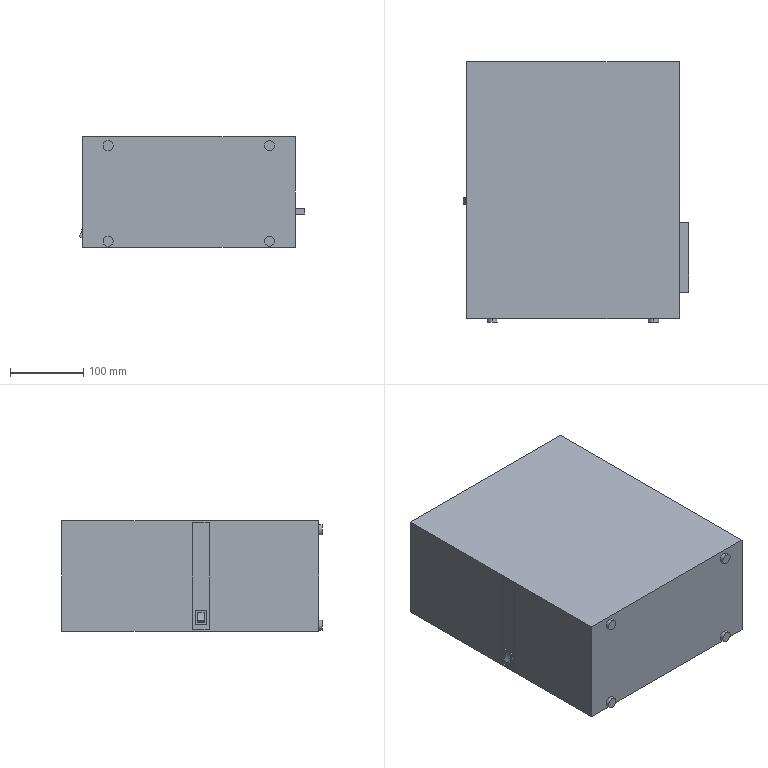Part | SolidWorks | features ICE 5, Extrusion 1 | 1 solid | 37 faces | box 307.5 x 355 x 150 mm | volume 15234035 mm3 | plane 28 | cylinder 9 | commonest cylinder face diameters 14 x8 44 x1
STEP:
#1=CARTESIAN_POINT('',(-110.,-5.,-74.));
#2=VERTEX_POINT('',#1);
#3=CARTESIAN_POINT('',(-110.,-5.,-60.));
#4=VERTEX_POINT('',#3);
#5=CARTESIAN_POINT('',(-110.,-5.,-67.));
#6=DIRECTION('',(0.,-1.,0.));
#7=DIRECTION('',(0.,0.,1.));
#8=AXIS2_PLACEMENT_3D('',#5,#6,#7);
#9=CIRCLE('',#8,7.);
#10=EDGE_CURVE('',#2,#4,#9,.T.);
#11=ORIENTED_EDGE('',*,*,#10,.F.);
#12=CARTESIAN_POINT('',(-110.,0.,-74.));
#13=VERTEX_POINT('',#12);
#14=CARTESIAN_POINT('',(-110.,-5.,-74.));
#15=DIRECTION('',(0.,1.,0.));
#16=VECTOR('',#15,1000.);
#17=LINE('',#14,#16);
#18=EDGE_CURVE('',#2,#13,#17,.T.);
#19=ORIENTED_EDGE('',*,*,#18,.T.);
#20=CARTESIAN_POINT('',(-110.,0.,-60.));
#21=VERTEX_POINT('',#20);
#22=CARTESIAN_POINT('',(-110.,0.,-67.));
#23=DIRECTION('',(0.,-1.,0.));
#24=DIRECTION('',(0.,0.,1.));
#25=AXIS2_PLACEMENT_3D('',#22,#23,#24);
#26=CIRCLE('',#25,7.);
#27=EDGE_CURVE('',#13,#21,#26,.T.);
#28=ORIENTED_EDGE('',*,*,#27,.T.);
#29=CARTESIAN_POINT('',(-110.,-5.,-60.));
#30=DIRECTION('',(0.,1.,0.));
#31=VECTOR('',#30,1000.);
#32=LINE('',#29,#31);
#33=EDGE_CURVE('',#4,#21,#32,.T.);
#34=ORIENTED_EDGE('',*,*,#33,.F.);
#35=EDGE_LOOP('',(#11,#19,#28,#34));
#36=FACE_OUTER_BOUND('',#35,.T.);
#37=CARTESIAN_POINT('',(-110.,-5.,-67.));
#38=DIRECTION('',(0.,1.,0.));
#39=DIRECTION('',(0.,0.,1.));
#40=AXIS2_PLACEMENT_3D('',#37,#38,#39);
#41=CYLINDRICAL_SURFACE('',#40,7.);
#42=ADVANCED_FACE('',(#36),#41,.T.);
#43=CARTESIAN_POINT('',(110.,-5.,-74.));
#44=VERTEX_POINT('',#43);
#45=CARTESIAN_POINT('',(110.,-5.,-60.));
#46=VERTEX_POINT('',#45);
#47=CARTESIAN_POINT('',(110.,-5.,-67.));
#48=DIRECTION('',(0.,-1.,0.));
#49=DIRECTION('',(0.,0.,-1.));
#50=AXIS2_PLACEMENT_3D('',#47,#48,#49);
#51=CIRCLE('',#50,7.);
#52=EDGE_CURVE('',#44,#46,#51,.T.);
#53=ORIENTED_EDGE('',*,*,#52,.F.);
#54=CARTESIAN_POINT('',(110.,0.,-74.));
#55=VERTEX_POINT('',#54);
#56=CARTESIAN_POINT('',(110.,-5.,-74.));
#57=DIRECTION('',(0.,1.,0.));
#58=VECTOR('',#57,1000.);
#59=LINE('',#56,#58);
#60=EDGE_CURVE('',#44,#55,#59,.T.);
#61=ORIENTED_EDGE('',*,*,#60,.T.);
#62=CARTESIAN_POINT('',(110.,0.,-60.));
#63=VERTEX_POINT('',#62);
#64=CARTESIAN_POINT('',(110.,0.,-67.));
#65=DIRECTION('',(0.,-1.,0.));
#66=DIRECTION('',(0.,0.,1.));
#67=AXIS2_PLACEMENT_3D('',#64,#65,#66);
#68=CIRCLE('',#67,7.);
#69=EDGE_CURVE('',#55,#63,#68,.T.);
#70=ORIENTED_EDGE('',*,*,#69,.T.);
#71=CARTESIAN_POINT('',(110.,-5.,-60.));
#72=DIRECTION('',(0.,1.,0.));
#73=VECTOR('',#72,1000.);
#74=LINE('',#71,#73);
#75=EDGE_CURVE('',#46,#63,#74,.T.);
#76=ORIENTED_EDGE('',*,*,#75,.F.);
#77=EDGE_LOOP('',(#53,#61,#70,#76));
#78=FACE_OUTER_BOUND('',#77,.T.);
#79=CARTESIAN_POINT('',(110.,-5.,-67.));
#80=DIRECTION('',(0.,1.,0.));
#81=DIRECTION('',(0.,0.,1.));
#82=AXIS2_PLACEMENT_3D('',#79,#80,#81);
#83=CYLINDRICAL_SURFACE('',#82,7.);
#84=ADVANCED_FACE('',(#78),#83,.T.);
#85=CARTESIAN_POINT('',(110.,-5.,56.));
#86=VERTEX_POINT('',#85);
#87=CARTESIAN_POINT('',(110.,-5.,70.));
#88=VERTEX_POINT('',#87);
#89=CARTESIAN_POINT('',(110.,-5.,63.));
#90=DIRECTION('',(0.,-1.,0.));
#91=DIRECTION('',(0.,0.,1.));
#92=AXIS2_PLACEMENT_3D('',#89,#90,#91);
#93=CIRCLE('',#92,7.);
#94=EDGE_CURVE('',#86,#88,#93,.T.);
#95=ORIENTED_EDGE('',*,*,#94,.F.);
#96=CARTESIAN_POINT('',(110.,0.,56.));
#97=VERTEX_POINT('',#96);
#98=CARTESIAN_POINT('',(110.,-5.,56.));
#99=DIRECTION('',(0.,1.,0.));
#100=VECTOR('',#99,1000.);
#101=LINE('',#98,#100);
#102=EDGE_CURVE('',#86,#97,#101,.T.);
#103=ORIENTED_EDGE('',*,*,#102,.T.);
#104=CARTESIAN_POINT('',(110.,0.,70.));
#105=VERTEX_POINT('',#104);
#106=CARTESIAN_POINT('',(110.,0.,63.));
#107=DIRECTION('',(0.,-1.,0.));
#108=DIRECTION('',(0.,0.,1.));
#109=AXIS2_PLACEMENT_3D('',#106,#107,#108);
#110=CIRCLE('',#109,7.);
#111=EDGE_CURVE('',#97,#105,#110,.T.);
#112=ORIENTED_EDGE('',*,*,#111,.T.);
#113=CARTESIAN_POINT('',(110.,-5.,70.));
#114=DIRECTION('',(0.,1.,0.));
#115=VECTOR('',#114,1000.);
#116=LINE('',#113,#115);
#117=EDGE_CURVE('',#88,#105,#116,.T.);
#118=ORIENTED_EDGE('',*,*,#117,.F.);
#119=EDGE_LOOP('',(#95,#103,#112,#118));
#120=FACE_OUTER_BOUND('',#119,.T.);
#121=CARTESIAN_POINT('',(110.,-5.,63.));
#122=DIRECTION('',(0.,1.,0.));
#123=DIRECTION('',(0.,0.,1.));
#124=AXIS2_PLACEMENT_3D('',#121,#122,#123);
#125=CYLINDRICAL_SURFACE('',#124,7.);
#126=ADVANCED_FACE('',(#120),#125,.T.);
#127=CARTESIAN_POINT('',(-110.,-5.,56.));
#128=VERTEX_POINT('',#127);
#129=CARTESIAN_POINT('',(-110.,-5.,70.));
#130=VERTEX_POINT('',#129);
#131=CARTESIAN_POINT('',(-110.,-5.,63.));
#132=DIRECTION('',(0.,-1.,0.));
#133=DIRECTION('',(0.,0.,-1.));
#134=AXIS2_PLACEMENT_3D('',#131,#132,#133);
#135=CIRCLE('',#134,7.);
#136=EDGE_CURVE('',#128,#130,#135,.T.);
#137=ORIENTED_EDGE('',*,*,#136,.F.);
#138=CARTESIAN_POINT('',(-110.,0.,56.));
#139=VERTEX_POINT('',#138);
#140=CARTESIAN_POINT('',(-110.,-5.,56.));
#141=DIRECTION('',(0.,1.,0.));
#142=VECTOR('',#141,1000.);
#143=LINE('',#140,#142);
#144=EDGE_CURVE('',#128,#139,#143,.T.);
#145=ORIENTED_EDGE('',*,*,#144,.T.);
#146=CARTESIAN_POINT('',(-110.,0.,70.));
#147=VERTEX_POINT('',#146);
#148=CARTESIAN_POINT('',(-110.,0.,63.));
#149=DIRECTION('',(0.,-1.,0.));
#150=DIRECTION('',(0.,0.,1.));
#151=AXIS2_PLACEMENT_3D('',#148,#149,#150);
#152=CIRCLE('',#151,7.);
#153=EDGE_CURVE('',#139,#147,#152,.T.);
#154=ORIENTED_EDGE('',*,*,#153,.T.);
#155=CARTESIAN_POINT('',(-110.,-5.,70.));
#156=DIRECTION('',(0.,1.,0.));
#157=VECTOR('',#156,1000.);
#158=LINE('',#155,#157);
#159=EDGE_CURVE('',#130,#147,#158,.T.);
#160=ORIENTED_EDGE('',*,*,#159,.F.);
#161=EDGE_LOOP('',(#137,#145,#154,#160));
#162=FACE_OUTER_BOUND('',#161,.T.);
#163=CARTESIAN_POINT('',(-110.,-5.,63.));
#164=DIRECTION('',(0.,1.,0.));
#165=DIRECTION('',(0.,0.,1.));
#166=AXIS2_PLACEMENT_3D('',#163,#164,#165);
#167=CYLINDRICAL_SURFACE('',#166,7.);
#168=ADVANCED_FACE('',(#162),#167,.T.);
#169=CARTESIAN_POINT('',(145.,0.,75.));
#170=VERTEX_POINT('',#169);
#171=CARTESIAN_POINT('',(145.,0.,-75.));
#172=VERTEX_POINT('',#171);
#173=CARTESIAN_POINT('',(145.,0.,75.));
#174=DIRECTION('',(0.,0.,-1.));
#175=VECTOR('',#174,1000.);
#176=LINE('',#173,#175);
#177=EDGE_CURVE('',#170,#172,#176,.T.);
#178=ORIENTED_EDGE('',*,*,#177,.T.);
#179=CARTESIAN_POINT('',(145.,350.,-75.));
#180=VERTEX_POINT('',#179);
#181=CARTESIAN_POINT('',(145.,350.,-75.));
#182=DIRECTION('',(0.,-1.,0.));
#183=VECTOR('',#182,1000.);
#184=LINE('',#181,#183);
#185=EDGE_CURVE('',#180,#172,#184,.T.);
#186=ORIENTED_EDGE('',*,*,#185,.F.);
#187=CARTESIAN_POINT('',(145.,350.,75.));
#188=VERTEX_POINT('',#187);
#189=CARTESIAN_POINT('',(145.,350.,75.));
#190=DIRECTION('',(0.,0.,-1.));
#191=VECTOR('',#190,1000.);
#192=LINE('',#189,#191);
#193=EDGE_CURVE('',#188,#180,#192,.T.);
#194=ORIENTED_EDGE('',*,*,#193,.F.);
#195=CARTESIAN_POINT('',(145.,350.,75.));
#196=DIRECTION('',(0.,-1.,0.));
#197=VECTOR('',#196,1000.);
#198=LINE('',#195,#197);
#199=EDGE_CURVE('',#188,#170,#198,.T.);
#200=ORIENTED_EDGE('',*,*,#199,.T.);
#201=EDGE_LOOP('',(#178,#186,#194,#200));
#202=FACE_OUTER_BOUND('',#201,.T.);
#203=CARTESIAN_POINT('',(145.,131.,-23.));
#204=VERTEX_POINT('',#203);
#205=CARTESIAN_POINT('',(145.,36.,-23.));
#206=VERTEX_POINT('',#205);
#207=CARTESIAN_POINT('',(145.,36.,-23.));
#208=DIRECTION('',(0.,-1.,0.));
#209=VECTOR('',#208,1000.);
#210=LINE('',#207,#209);
#211=EDGE_CURVE('',#204,#206,#210,.T.);
#212=ORIENTED_EDGE('',*,*,#211,.F.);
#213=CARTESIAN_POINT('',(145.,131.,-30.));
#214=VERTEX_POINT('',#213);
#215=CARTESIAN_POINT('',(145.,131.,-30.));
#216=DIRECTION('',(0.,0.,1.));
#217=VECTOR('',#216,1000.);
#218=LINE('',#215,#217);
#219=EDGE_CURVE('',#214,#204,#218,.T.);
#220=ORIENTED_EDGE('',*,*,#219,.F.);
#221=CARTESIAN_POINT('',(145.,36.,-30.));
#222=VERTEX_POINT('',#221);
#223=CARTESIAN_POINT('',(145.,36.,-30.));
#224=DIRECTION('',(0.,1.,0.));
#225=VECTOR('',#224,1000.);
#226=LINE('',#223,#225);
#227=EDGE_CURVE('',#222,#214,#226,.T.);
#228=ORIENTED_EDGE('',*,*,#227,.F.);
#229=CARTESIAN_POINT('',(145.,36.,-30.));
#230=DIRECTION('',(0.,0.,-1.));
#231=VECTOR('',#230,1000.);
#232=LINE('',#229,#231);
#233=EDGE_CURVE('',#206,#222,#232,.T.);
#234=ORIENTED_EDGE('',*,*,#233,.F.);
#235=EDGE_LOOP('',(#212,#220,#228,#234));
#236=FACE_BOUND('',#235,.T.);
#237=CARTESIAN_POINT('',(145.,350.,75.));
#238=DIRECTION('',(-1.,0.,0.));
#239=DIRECTION('',(0.,0.,1.));
#240=AXIS2_PLACEMENT_3D('',#237,#238,#239);
#241=PLANE('',#240);
#242=ADVANCED_FACE('',(#202,#236),#241,.F.);
#243=CARTESIAN_POINT('',(-145.5,168.,-66.5));
#244=VERTEX_POINT('',#243);
#245=CARTESIAN_POINT('',(-145.5,153.,-66.5));
#246=VERTEX_POINT('',#245);
#247=CARTESIAN_POINT('',(-145.5,153.,-66.5));
#248=DIRECTION('',(0.,-1.,0.));
#249=VECTOR('',#248,1000.);
#250=LINE('',#247,#249);
#251=EDGE_CURVE('',#244,#246,#250,.T.);
#252=ORIENTED_EDGE('',*,*,#251,.T.);
#253=CARTESIAN_POINT('',(-145.5,153.,-46.5));
#254=VERTEX_POINT('',#253);
#255=CARTESIAN_POINT('',(-145.5,153.,-46.5));
#256=DIRECTION('',(0.,0.,1.));
#257=VECTOR('',#256,1000.);
#258=LINE('',#255,#257);
#259=EDGE_CURVE('',#246,#254,#258,.T.);
#260=ORIENTED_EDGE('',*,*,#259,.T.);
#261=CARTESIAN_POINT('',(-145.5,168.,-46.5));
#262=VERTEX_POINT('',#261);
#263=CARTESIAN_POINT('',(-145.5,153.,-46.5));
#264=DIRECTION('',(0.,1.,0.));
#265=VECTOR('',#264,1000.);
#266=LINE('',#263,#265);
#267=EDGE_CURVE('',#254,#262,#266,.T.);
#268=ORIENTED_EDGE('',*,*,#267,.T.);
#269=CARTESIAN_POINT('',(-145.5,168.,-46.5));
#270=DIRECTION('',(0.,0.,-1.));
#271=VECTOR('',#270,1000.);
#272=LINE('',#269,#271);
#273=EDGE_CURVE('',#262,#244,#272,.T.);
#274=ORIENTED_EDGE('',*,*,#273,.T.);
#275=EDGE_LOOP('',(#252,#260,#268,#274));
#276=FACE_OUTER_BOUND('',#275,.T.);
#277=CARTESIAN_POINT('',(-145.5,156.,-49.5));
#278=VERTEX_POINT('',#277);
#279=CARTESIAN_POINT('',(-145.5,165.,-49.5));
#280=VERTEX_POINT('',#279);
#281=CARTESIAN_POINT('',(-145.5,156.,-49.5));
#282=DIRECTION('',(0.,1.,0.));
#283=VECTOR('',#282,1000.);
#284=LINE('',#281,#283);
#285=EDGE_CURVE('',#278,#280,#284,.T.);
#286=ORIENTED_EDGE('',*,*,#285,.F.);
#287=CARTESIAN_POINT('',(-145.5,156.,-63.5));
#288=VERTEX_POINT('',#287);
#289=CARTESIAN_POINT('',(-145.5,156.,-63.5));
#290=DIRECTION('',(0.,0.,1.));
#291=VECTOR('',#290,1000.);
#292=LINE('',#289,#291);
#293=EDGE_CURVE('',#288,#278,#292,.T.);
#294=ORIENTED_EDGE('',*,*,#293,.F.);
#295=CARTESIAN_POINT('',(-145.5,165.,-63.5));
#296=VERTEX_POINT('',#295);
#297=CARTESIAN_POINT('',(-145.5,156.,-63.5));
#298=DIRECTION('',(0.,1.,0.));
#299=VECTOR('',#298,1000.);
#300=LINE('',#297,#299);
#301=EDGE_CURVE('',#288,#296,#300,.T.);
#302=ORIENTED_EDGE('',*,*,#301,.T.);
#303=CARTESIAN_POINT('',(-145.5,165.,-63.5));
#304=DIRECTION('',(0.,0.,1.));
#305=VECTOR('',#304,1000.);
#306=LINE('',#303,#305);
#307=EDGE_CURVE('',#296,#280,#306,.T.);
#308=ORIENTED_EDGE('',*,*,#307,.T.);
#309=EDGE_LOOP('',(#286,#294,#302,#308));
#310=FACE_BOUND('',#309,.T.);
#311=CARTESIAN_POINT('',(-145.5,0.,0.));
#312=DIRECTION('',(-1.,0.,0.));
#313=DIRECTION('',(0.,0.,1.));
#314=AXIS2_PLACEMENT_3D('',#311,#312,#313);
#315=PLANE('',#314);
#316=ADVANCED_FACE('',(#276,#310),#315,.T.);
#317=CARTESIAN_POINT('',(-144.,172.,-72.5));
#318=VERTEX_POINT('',#317);
#319=CARTESIAN_POINT('',(-144.,149.,-72.5));
#320=VERTEX_POINT('',#319);
#321=CARTESIAN_POINT('',(-144.,149.,-72.5));
#322=DIRECTION('',(0.,-1.,0.));
#323=VECTOR('',#322,1000.);
#324=LINE('',#321,#323);
#325=EDGE_CURVE('',#318,#320,#324,.T.);
#326=ORIENTED_EDGE('',*,*,#325,.T.);
#327=CARTESIAN_POINT('',(-144.,149.,72.5));
#328=VERTEX_POINT('',#327);
#329=CARTESIAN_POINT('',(-144.,149.,72.5));
#330=DIRECTION('',(0.,0.,1.));
#331=VECTOR('',#330,1000.);
#332=LINE('',#329,#331);
#333=EDGE_CURVE('',#320,#328,#332,.T.);
#334=ORIENTED_EDGE('',*,*,#333,.T.);
#335=CARTESIAN_POINT('',(-144.,172.,72.5));
#336=VERTEX_POINT('',#335);
#337=CARTESIAN_POINT('',(-144.,149.,72.5));
#338=DIRECTION('',(0.,1.,0.));
#339=VECTOR('',#338,1000.);
#340=LINE('',#337,#339);
#341=EDGE_CURVE('',#328,#336,#340,.T.);
#342=ORIENTED_EDGE('',*,*,#341,.T.);
#343=CARTESIAN_POINT('',(-144.,172.,72.5));
#344=DIRECTION('',(0.,0.,-1.));
#345=VECTOR('',#344,1000.);
#346=LINE('',#343,#345);
#347=EDGE_CURVE('',#336,#318,#346,.T.);
#348=ORIENTED_EDGE('',*,*,#347,.T.);
#349=EDGE_LOOP('',(#326,#334,#342,#348));
#350=FACE_OUTER_BOUND('',#349,.T.);
#351=CARTESIAN_POINT('',(-144.,153.,-66.5));
#352=VERTEX_POINT('',#351);
#353=CARTESIAN_POINT('',(-144.,153.,-46.5));
#354=VERTEX_POINT('',#353);
#355=CARTESIAN_POINT('',(-144.,153.,-46.5));
#356=DIRECTION('',(0.,0.,1.));
#357=VECTOR('',#356,1000.);
#358=LINE('',#355,#357);
#359=EDGE_CURVE('',#352,#354,#358,.T.);
#360=ORIENTED_EDGE('',*,*,#359,.F.);
#361=CARTESIAN_POINT('',(-144.,168.,-66.5));
#362=VERTEX_POINT('',#361);
#363=CARTESIAN_POINT('',(-144.,153.,-66.5));
#364=DIRECTION('',(0.,-1.,0.));
#365=VECTOR('',#364,1000.);
#366=LINE('',#363,#365);
#367=EDGE_CURVE('',#362,#352,#366,.T.);
#368=ORIENTED_EDGE('',*,*,#367,.F.);
#369=CARTESIAN_POINT('',(-144.,168.,-46.5));
#370=VERTEX_POINT('',#369);
#371=CARTESIAN_POINT('',(-144.,168.,-46.5));
#372=DIRECTION('',(0.,0.,-1.));
#373=VECTOR('',#372,1000.);
#374=LINE('',#371,#373);
#375=EDGE_CURVE('',#370,#362,#374,.T.);
#376=ORIENTED_EDGE('',*,*,#375,.F.);
#377=CARTESIAN_POINT('',(-144.,153.,-46.5));
#378=DIRECTION('',(0.,1.,0.));
#379=VECTOR('',#378,1000.);
#380=LINE('',#377,#379);
#381=EDGE_CURVE('',#354,#370,#380,.T.);
#382=ORIENTED_EDGE('',*,*,#381,.F.);
#383=EDGE_LOOP('',(#360,#368,#376,#382));
#384=FACE_BOUND('',#383,.T.);
#385=CARTESIAN_POINT('',(-144.,0.,0.));
#386=DIRECTION('',(-1.,0.,0.));
#387=DIRECTION('',(0.,0.,1.));
#388=AXIS2_PLACEMENT_3D('',#385,#386,#387);
#389=PLANE('',#388);
#390=ADVANCED_FACE('',(#350,#384),#389,.T.);
#391=CARTESIAN_POINT('',(-145.,149.,-72.5));
#392=VERTEX_POINT('',#391);
#393=CARTESIAN_POINT('',(-145.,149.,72.5));
#394=VERTEX_POINT('',#393);
#395=CARTESIAN_POINT('',(-145.,149.,72.5));
#396=DIRECTION('',(0.,0.,1.));
#397=VECTOR('',#396,1000.);
#398=LINE('',#395,#397);
#399=EDGE_CURVE('',#392,#394,#398,.T.);
#400=ORIENTED_EDGE('',*,*,#399,.F.);
#401=CARTESIAN_POINT('',(-145.,172.,-72.5));
#402=VERTEX_POINT('',#401);
#403=CARTESIAN_POINT('',(-145.,149.,-72.5));
#404=DIRECTION('',(0.,-1.,0.));
#405=VECTOR('',#404,1000.);
#406=LINE('',#403,#405);
#407=EDGE_CURVE('',#402,#392,#406,.T.);
#408=ORIENTED_EDGE('',*,*,#407,.F.);
#409=CARTESIAN_POINT('',(-145.,172.,72.5));
#410=VERTEX_POINT('',#409);
#411=CARTESIAN_POINT('',(-145.,172.,72.5));
#412=DIRECTION('',(0.,0.,-1.));
#413=VECTOR('',#412,1000.);
#414=LINE('',#411,#413);
#415=EDGE_CURVE('',#410,#402,#414,.T.);
#416=ORIENTED_EDGE('',*,*,#415,.F.);
#417=CARTESIAN_POINT('',(-145.,149.,72.5));
#418=DIRECTION('',(0.,1.,0.));
#419=VECTOR('',#418,1000.);
#420=LINE('',#417,#419);
#421=EDGE_CURVE('',#394,#410,#420,.T.);
#422=ORIENTED_EDGE('',*,*,#421,.F.);
#423=EDGE_LOOP('',(#400,#408,#416,#422));
#424=FACE_BOUND('',#423,.T.);
#425=CARTESIAN_POINT('',(-145.,0.,-75.));
#426=VERTEX_POINT('',#425);
#427=CARTESIAN_POINT('',(-145.,0.,75.));
#428=VERTEX_POINT('',#427);
#429=CARTESIAN_POINT('',(-145.,0.,75.));
#430=DIRECTION('',(0.,0.,1.));
#431=VECTOR('',#430,1000.);
#432=LINE('',#429,#431);
#433=EDGE_CURVE('',#426,#428,#432,.T.);
#434=ORIENTED_EDGE('',*,*,#433,.T.);
#435=CARTESIAN_POINT('',(-145.,350.,75.));
#436=VERTEX_POINT('',#435);
#437=CARTESIAN_POINT('',(-145.,350.,75.));
#438=DIRECTION('',(0.,-1.,0.));
#439=VECTOR('',#438,1000.);
#440=LINE('',#437,#439);
#441=EDGE_CURVE('',#436,#428,#440,.T.);
#442=ORIENTED_EDGE('',*,*,#441,.F.);
#443=CARTESIAN_POINT('',(-145.,350.,-75.));
#444=VERTEX_POINT('',#443);
#445=CARTESIAN_POINT('',(-145.,350.,75.));
#446=DIRECTION('',(0.,0.,1.));
#447=VECTOR('',#446,1000.);
#448=LINE('',#445,#447);
#449=EDGE_CURVE('',#444,#436,#448,.T.);
#450=ORIENTED_EDGE('',*,*,#449,.F.);
#451=CARTESIAN_POINT('',(-145.,350.,-75.));
#452=DIRECTION('',(0.,-1.,0.));
#453=VECTOR('',#452,1000.);
#454=LINE('',#451,#453);
#455=EDGE_CURVE('',#444,#426,#454,.T.);
#456=ORIENTED_EDGE('',*,*,#455,.T.);
#457=EDGE_LOOP('',(#434,#442,#450,#456));
#458=FACE_OUTER_BOUND('',#457,.T.);
#459=CARTESIAN_POINT('',(-145.,350.,75.));
#460=DIRECTION('',(1.,0.,0.));
#461=DIRECTION('',(0.,0.,-1.));
#462=AXIS2_PLACEMENT_3D('',#459,#460,#461);
#463=PLANE('',#462);
#464=ADVANCED_FACE('',(#424,#458),#463,.F.);
#465=CARTESIAN_POINT('',(145.,0.,75.));
#466=DIRECTION('',(1.,0.,0.));
#467=VECTOR('',#466,1000.);
#468=LINE('',#465,#467);
#469=EDGE_CURVE('',#428,#170,#468,.T.);
#470=ORIENTED_EDGE('',*,*,#469,.T.);
#471=ORIENTED_EDGE('',*,*,#199,.F.);
#472=CARTESIAN_POINT('',(145.,350.,75.));
#473=DIRECTION('',(1.,0.,0.));
#474=VECTOR('',#473,1000.);
#475=LINE('',#472,#474);
#476=EDGE_CURVE('',#436,#188,#475,.T.);
#477=ORIENTED_EDGE('',*,*,#476,.F.);
#478=ORIENTED_EDGE('',*,*,#441,.T.);
#479=EDGE_LOOP('',(#470,#471,#477,#478));
#480=FACE_OUTER_BOUND('',#479,.T.);
#481=CARTESIAN_POINT('',(145.,350.,75.));
#482=DIRECTION('',(0.,0.,-1.));
#483=DIRECTION('',(-1.,0.,0.));
#484=AXIS2_PLACEMENT_3D('',#481,#482,#483);
#485=PLANE('',#484);
#486=ADVANCED_FACE('',(#480),#485,.F.);
#487=CARTESIAN_POINT('',(145.,0.,-75.));
#488=DIRECTION('',(-1.,0.,0.));
#489=VECTOR('',#488,1000.);
#490=LINE('',#487,#489);
#491=EDGE_CURVE('',#172,#426,#490,.T.);
#492=ORIENTED_EDGE('',*,*,#491,.T.);
#493=ORIENTED_EDGE('',*,*,#455,.F.);
#494=CARTESIAN_POINT('',(145.,350.,-75.));
#495=DIRECTION('',(-1.,0.,0.));
#496=VECTOR('',#495,1000.);
#497=LINE('',#494,#496);
#498=EDGE_CURVE('',#180,#444,#497,.T.);
#499=ORIENTED_EDGE('',*,*,#498,.F.);
#500=ORIENTED_EDGE('',*,*,#185,.T.);
#501=EDGE_LOOP('',(#492,#493,#499,#500));
#502=FACE_OUTER_BOUND('',#501,.T.);
#503=CARTESIAN_POINT('',(145.,350.,-75.));
#504=DIRECTION('',(0.,0.,1.));
#505=DIRECTION('',(1.,0.,0.));
#506=AXIS2_PLACEMENT_3D('',#503,#504,#505);
#507=PLANE('',#506);
#508=ADVANCED_FACE('',(#502),#507,.F.);
#509=ORIENTED_EDGE('',*,*,#449,.T.);
#510=ORIENTED_EDGE('',*,*,#476,.T.);
#511=ORIENTED_EDGE('',*,*,#193,.T.);
#512=ORIENTED_EDGE('',*,*,#498,.T.);
#513=EDGE_LOOP('',(#509,#510,#511,#512));
#514=FACE_OUTER_BOUND('',#513,.T.);
#515=CARTESIAN_POINT('',(0.,350.,0.));
#516=DIRECTION('',(0.,1.,0.));
#517=DIRECTION('',(0.,0.,1.));
#518=AXIS2_PLACEMENT_3D('',#515,#516,#517);
#519=PLANE('',#518);
#520=ADVANCED_FACE('',(#514),#519,.T.);
#521=CARTESIAN_POINT('',(-110.,0.,-67.));
#522=DIRECTION('',(0.,-1.,0.));
#523=DIRECTION('',(0.,0.,1.));
#524=AXIS2_PLACEMENT_3D('',#521,#522,#523);
#525=CIRCLE('',#524,7.);
#526=EDGE_CURVE('',#21,#13,#525,.T.);
#527=ORIENTED_EDGE('',*,*,#526,.F.);
#528=ORIENTED_EDGE('',*,*,#27,.F.);
#529=EDGE_LOOP('',(#527,#528));
#530=FACE_BOUND('',#529,.T.);
#531=CARTESIAN_POINT('',(110.,0.,-67.));
#532=DIRECTION('',(0.,-1.,0.));
#533=DIRECTION('',(0.,0.,1.));
#534=AXIS2_PLACEMENT_3D('',#531,#532,#533);
#535=CIRCLE('',#534,7.);
#536=EDGE_CURVE('',#63,#55,#535,.T.);
#537=ORIENTED_EDGE('',*,*,#536,.F.);
#538=ORIENTED_EDGE('',*,*,#69,.F.);
#539=EDGE_LOOP('',(#537,#538));
#540=FACE_BOUND('',#539,.T.);
#541=CARTESIAN_POINT('',(110.,0.,63.));
#542=DIRECTION('',(0.,-1.,0.));
#543=DIRECTION('',(0.,0.,1.));
#544=AXIS2_PLACEMENT_3D('',#541,#542,#543);
#545=CIRCLE('',#544,7.);
#546=EDGE_CURVE('',#105,#97,#545,.T.);
#547=ORIENTED_EDGE('',*,*,#546,.F.);
#548=ORIENTED_EDGE('',*,*,#111,.F.);
#549=EDGE_LOOP('',(#547,#548));
#550=FACE_BOUND('',#549,.T.);
#551=CARTESIAN_POINT('',(-110.,0.,63.));
#552=DIRECTION('',(0.,-1.,0.));
#553=DIRECTION('',(0.,0.,1.));
#554=AXIS2_PLACEMENT_3D('',#551,#552,#553);
#555=CIRCLE('',#554,7.);
#556=EDGE_CURVE('',#147,#139,#555,.T.);
#557=ORIENTED_EDGE('',*,*,#556,.F.);
#558=ORIENTED_EDGE('',*,*,#153,.F.);
#559=EDGE_LOOP('',(#557,#558));
#560=FACE_BOUND('',#559,.T.);
#561=ORIENTED_EDGE('',*,*,#433,.F.);
#562=ORIENTED_EDGE('',*,*,#491,.F.);
#563=ORIENTED_EDGE('',*,*,#177,.F.);
#564=ORIENTED_EDGE('',*,*,#469,.F.);
#565=EDGE_LOOP('',(#561,#562,#563,#564));
#566=FACE_OUTER_BOUND('',#565,.T.);
#567=CARTESIAN_POINT('',(0.,0.,0.));
#568=DIRECTION('',(0.,1.,0.));
#569=DIRECTION('',(0.,0.,1.));
#570=AXIS2_PLACEMENT_3D('',#567,#568,#569);
#571=PLANE('',#570);
#572=ADVANCED_FACE('',(#530,#540,#550,#560,#566),#571,.F.);
#573=ORIENTED_EDGE('',*,*,#144,.F.);
#574=CARTESIAN_POINT('',(-110.,-5.,63.));
#575=DIRECTION('',(0.,-1.,0.));
#576=DIRECTION('',(0.,0.,-1.));
#577=AXIS2_PLACEMENT_3D('',#574,#575,#576);
#578=CIRCLE('',#577,7.);
#579=EDGE_CURVE('',#130,#128,#578,.T.);
#580=ORIENTED_EDGE('',*,*,#579,.F.);
#581=ORIENTED_EDGE('',*,*,#159,.T.);
#582=ORIENTED_EDGE('',*,*,#556,.T.);
#583=EDGE_LOOP('',(#573,#580,#581,#582));
#584=FACE_OUTER_BOUND('',#583,.T.);
#585=CARTESIAN_POINT('',(-110.,-5.,63.));
#586=DIRECTION('',(0.,1.,0.));
#587=DIRECTION('',(0.,0.,1.));
#588=AXIS2_PLACEMENT_3D('',#585,#586,#587);
#589=CYLINDRICAL_SURFACE('',#588,7.);
#590=ADVANCED_FACE('',(#584),#589,.T.);
#591=ORIENTED_EDGE('',*,*,#579,.T.);
#592=ORIENTED_EDGE('',*,*,#136,.T.);
#593=EDGE_LOOP('',(#591,#592));
#594=FACE_OUTER_BOUND('',#593,.T.);
#595=CARTESIAN_POINT('',(-110.,-5.,63.));
#596=DIRECTION('',(0.,-1.,0.));
#597=DIRECTION('',(0.,0.,-1.));
#598=AXIS2_PLACEMENT_3D('',#595,#596,#597);
#599=PLANE('',#598);
#600=ADVANCED_FACE('',(#594),#599,.T.);
#601=ORIENTED_EDGE('',*,*,#102,.F.);
#602=CARTESIAN_POINT('',(110.,-5.,63.));
#603=DIRECTION('',(0.,-1.,0.));
#604=DIRECTION('',(0.,0.,1.));
#605=AXIS2_PLACEMENT_3D('',#602,#603,#604);
#606=CIRCLE('',#605,7.);
#607=EDGE_CURVE('',#88,#86,#606,.T.);
#608=ORIENTED_EDGE('',*,*,#607,.F.);
#609=ORIENTED_EDGE('',*,*,#117,.T.);
#610=ORIENTED_EDGE('',*,*,#546,.T.);
#611=EDGE_LOOP('',(#601,#608,#609,#610));
#612=FACE_OUTER_BOUND('',#611,.T.);
#613=CARTESIAN_POINT('',(110.,-5.,63.));
#614=DIRECTION('',(0.,1.,0.));
#615=DIRECTION('',(0.,0.,1.));
#616=AXIS2_PLACEMENT_3D('',#613,#614,#615);
#617=CYLINDRICAL_SURFACE('',#616,7.);
#618=ADVANCED_FACE('',(#612),#617,.T.);
#619=ORIENTED_EDGE('',*,*,#607,.T.);
#620=ORIENTED_EDGE('',*,*,#94,.T.);
#621=EDGE_LOOP('',(#619,#620));
#622=FACE_OUTER_BOUND('',#621,.T.);
#623=CARTESIAN_POINT('',(110.,-5.,63.));
#624=DIRECTION('',(0.,1.,0.));
#625=DIRECTION('',(0.,0.,1.));
#626=AXIS2_PLACEMENT_3D('',#623,#624,#625);
#627=PLANE('',#626);
#628=ADVANCED_FACE('',(#622),#627,.F.);
#629=ORIENTED_EDGE('',*,*,#60,.F.);
#630=CARTESIAN_POINT('',(110.,-5.,-67.));
#631=DIRECTION('',(0.,-1.,0.));
#632=DIRECTION('',(0.,0.,-1.));
#633=AXIS2_PLACEMENT_3D('',#630,#631,#632);
#634=CIRCLE('',#633,7.);
#635=EDGE_CURVE('',#46,#44,#634,.T.);
#636=ORIENTED_EDGE('',*,*,#635,.F.);
#637=ORIENTED_EDGE('',*,*,#75,.T.);
#638=ORIENTED_EDGE('',*,*,#536,.T.);
#639=EDGE_LOOP('',(#629,#636,#637,#638));
#640=FACE_OUTER_BOUND('',#639,.T.);
#641=CARTESIAN_POINT('',(110.,-5.,-67.));
#642=DIRECTION('',(0.,1.,0.));
#643=DIRECTION('',(0.,0.,1.));
#644=AXIS2_PLACEMENT_3D('',#641,#642,#643);
#645=CYLINDRICAL_SURFACE('',#644,7.);
#646=ADVANCED_FACE('',(#640),#645,.T.);
#647=ORIENTED_EDGE('',*,*,#635,.T.);
#648=ORIENTED_EDGE('',*,*,#52,.T.);
#649=EDGE_LOOP('',(#647,#648));
#650=FACE_OUTER_BOUND('',#649,.T.);
#651=CARTESIAN_POINT('',(110.,-5.,-67.));
#652=DIRECTION('',(0.,-1.,0.));
#653=DIRECTION('',(0.,0.,-1.));
#654=AXIS2_PLACEMENT_3D('',#651,#652,#653);
#655=PLANE('',#654);
#656=ADVANCED_FACE('',(#650),#655,.T.);
#657=ORIENTED_EDGE('',*,*,#18,.F.);
#658=CARTESIAN_POINT('',(-110.,-5.,-67.));
#659=DIRECTION('',(0.,-1.,0.));
#660=DIRECTION('',(0.,0.,1.));
#661=AXIS2_PLACEMENT_3D('',#658,#659,#660);
#662=CIRCLE('',#661,7.);
#663=EDGE_CURVE('',#4,#2,#662,.T.);
#664=ORIENTED_EDGE('',*,*,#663,.F.);
#665=ORIENTED_EDGE('',*,*,#33,.T.);
#666=ORIENTED_EDGE('',*,*,#526,.T.);
#667=EDGE_LOOP('',(#657,#664,#665,#666));
#668=FACE_OUTER_BOUND('',#667,.T.);
#669=CARTESIAN_POINT('',(-110.,-5.,-67.));
#670=DIRECTION('',(0.,1.,0.));
#671=DIRECTION('',(0.,0.,1.));
#672=AXIS2_PLACEMENT_3D('',#669,#670,#671);
#673=CYLINDRICAL_SURFACE('',#672,7.);
#674=ADVANCED_FACE('',(#668),#673,.T.);
#675=ORIENTED_EDGE('',*,*,#663,.T.);
#676=ORIENTED_EDGE('',*,*,#10,.T.);
#677=EDGE_LOOP('',(#675,#676));
#678=FACE_OUTER_BOUND('',#677,.T.);
#679=CARTESIAN_POINT('',(-110.,-5.,-67.));
#680=DIRECTION('',(0.,1.,0.));
#681=DIRECTION('',(0.,0.,1.));
#682=AXIS2_PLACEMENT_3D('',#679,#680,#681);
#683=PLANE('',#682);
#684=ADVANCED_FACE('',(#678),#683,.F.);
#685=ORIENTED_EDGE('',*,*,#407,.T.);
#686=CARTESIAN_POINT('',(-144.,149.,-72.5));
#687=DIRECTION('',(-1.,0.,0.));
#688=VECTOR('',#687,1000.);
#689=LINE('',#686,#688);
#690=EDGE_CURVE('',#320,#392,#689,.T.);
#691=ORIENTED_EDGE('',*,*,#690,.F.);
#692=ORIENTED_EDGE('',*,*,#325,.F.);
#693=CARTESIAN_POINT('',(-144.,172.,-72.5));
#694=DIRECTION('',(-1.,0.,0.));
#695=VECTOR('',#694,1000.);
#696=LINE('',#693,#695);
#697=EDGE_CURVE('',#318,#402,#696,.T.);
#698=ORIENTED_EDGE('',*,*,#697,.T.);
#699=EDGE_LOOP('',(#685,#691,#692,#698));
#700=FACE_OUTER_BOUND('',#699,.T.);
#701=CARTESIAN_POINT('',(-144.,149.,-72.5));
#702=DIRECTION('',(0.,0.,-1.));
#703=DIRECTION('',(-1.,0.,0.));
#704=AXIS2_PLACEMENT_3D('',#701,#702,#703);
#705=PLANE('',#704);
#706=ADVANCED_FACE('',(#700),#705,.F.);
#707=ORIENTED_EDGE('',*,*,#415,.T.);
#708=ORIENTED_EDGE('',*,*,#697,.F.);
#709=ORIENTED_EDGE('',*,*,#347,.F.);
#710=CARTESIAN_POINT('',(-144.,172.,72.5));
#711=DIRECTION('',(-1.,0.,0.));
#712=VECTOR('',#711,1000.);
#713=LINE('',#710,#712);
#714=EDGE_CURVE('',#336,#410,#713,.T.);
#715=ORIENTED_EDGE('',*,*,#714,.T.);
#716=EDGE_LOOP('',(#707,#708,#709,#715));
#717=FACE_OUTER_BOUND('',#716,.T.);
#718=CARTESIAN_POINT('',(-144.,172.,72.5));
#719=DIRECTION('',(0.,1.,0.));
#720=DIRECTION('',(0.,0.,1.));
#721=AXIS2_PLACEMENT_3D('',#718,#719,#720);
#722=PLANE('',#721);
#723=ADVANCED_FACE('',(#717),#722,.F.);
#724=ORIENTED_EDGE('',*,*,#421,.T.);
#725=ORIENTED_EDGE('',*,*,#714,.F.);
#726=ORIENTED_EDGE('',*,*,#341,.F.);
#727=CARTESIAN_POINT('',(-144.,149.,72.5));
#728=DIRECTION('',(-1.,0.,0.));
#729=VECTOR('',#728,1000.);
#730=LINE('',#727,#729);
#731=EDGE_CURVE('',#328,#394,#730,.T.);
#732=ORIENTED_EDGE('',*,*,#731,.T.);
#733=EDGE_LOOP('',(#724,#725,#726,#732));
#734=FACE_OUTER_BOUND('',#733,.T.);
#735=CARTESIAN_POINT('',(-144.,149.,72.5));
#736=DIRECTION('',(0.,0.,1.));
#737=DIRECTION('',(1.,0.,0.));
#738=AXIS2_PLACEMENT_3D('',#735,#736,#737);
#739=PLANE('',#738);
#740=ADVANCED_FACE('',(#734),#739,.F.);
#741=ORIENTED_EDGE('',*,*,#399,.T.);
#742=ORIENTED_EDGE('',*,*,#731,.F.);
#743=ORIENTED_EDGE('',*,*,#333,.F.);
#744=ORIENTED_EDGE('',*,*,#690,.T.);
#745=EDGE_LOOP('',(#741,#742,#743,#744));
#746=FACE_OUTER_BOUND('',#745,.T.);
#747=CARTESIAN_POINT('',(-144.,149.,72.5));
#748=DIRECTION('',(0.,-1.,0.));
#749=DIRECTION('',(0.,0.,-1.));
#750=AXIS2_PLACEMENT_3D('',#747,#748,#749);
#751=PLANE('',#750);
#752=ADVANCED_FACE('',(#746),#751,.F.);
#753=ORIENTED_EDGE('',*,*,#367,.T.);
#754=CARTESIAN_POINT('',(-145.5,153.,-66.5));
#755=DIRECTION('',(1.,0.,0.));
#756=VECTOR('',#755,1000.);
#757=LINE('',#754,#756);
#758=EDGE_CURVE('',#246,#352,#757,.T.);
#759=ORIENTED_EDGE('',*,*,#758,.F.);
#760=ORIENTED_EDGE('',*,*,#251,.F.);
#761=CARTESIAN_POINT('',(-145.5,168.,-66.5));
#762=DIRECTION('',(1.,0.,0.));
#763=VECTOR('',#762,1000.);
#764=LINE('',#761,#763);
#765=EDGE_CURVE('',#244,#362,#764,.T.);
#766=ORIENTED_EDGE('',*,*,#765,.T.);
#767=EDGE_LOOP('',(#753,#759,#760,#766));
#768=FACE_OUTER_BOUND('',#767,.T.);
#769=CARTESIAN_POINT('',(-145.5,153.,-66.5));
#770=DIRECTION('',(0.,0.,1.));
#771=DIRECTION('',(1.,0.,0.));
#772=AXIS2_PLACEMENT_3D('',#769,#770,#771);
#773=PLANE('',#772);
#774=ADVANCED_FACE('',(#768),#773,.F.);
#775=ORIENTED_EDGE('',*,*,#359,.T.);
#776=CARTESIAN_POINT('',(-145.5,153.,-46.5));
#777=DIRECTION('',(1.,0.,0.));
#778=VECTOR('',#777,1000.);
#779=LINE('',#776,#778);
#780=EDGE_CURVE('',#254,#354,#779,.T.);
#781=ORIENTED_EDGE('',*,*,#780,.F.);
#782=ORIENTED_EDGE('',*,*,#259,.F.);
#783=ORIENTED_EDGE('',*,*,#758,.T.);
#784=EDGE_LOOP('',(#775,#781,#782,#783));
#785=FACE_OUTER_BOUND('',#784,.T.);
#786=CARTESIAN_POINT('',(-145.5,153.,-46.5));
#787=DIRECTION('',(0.,1.,0.));
#788=DIRECTION('',(0.,0.,1.));
#789=AXIS2_PLACEMENT_3D('',#786,#787,#788);
#790=PLANE('',#789);
#791=ADVANCED_FACE('',(#785),#790,.F.);
#792=ORIENTED_EDGE('',*,*,#381,.T.);
#793=CARTESIAN_POINT('',(-145.5,168.,-46.5));
#794=DIRECTION('',(1.,0.,0.));
#795=VECTOR('',#794,1000.);
#796=LINE('',#793,#795);
#797=EDGE_CURVE('',#262,#370,#796,.T.);
#798=ORIENTED_EDGE('',*,*,#797,.F.);
#799=ORIENTED_EDGE('',*,*,#267,.F.);
#800=ORIENTED_EDGE('',*,*,#780,.T.);
#801=EDGE_LOOP('',(#792,#798,#799,#800));
#802=FACE_OUTER_BOUND('',#801,.T.);
#803=CARTESIAN_POINT('',(-145.5,153.,-46.5));
#804=DIRECTION('',(0.,0.,-1.));
#805=DIRECTION('',(-1.,0.,0.));
#806=AXIS2_PLACEMENT_3D('',#803,#804,#805);
#807=PLANE('',#806);
#808=ADVANCED_FACE('',(#802),#807,.F.);
#809=ORIENTED_EDGE('',*,*,#375,.T.);
#810=ORIENTED_EDGE('',*,*,#765,.F.);
#811=ORIENTED_EDGE('',*,*,#273,.F.);
#812=ORIENTED_EDGE('',*,*,#797,.T.);
#813=EDGE_LOOP('',(#809,#810,#811,#812));
#814=FACE_OUTER_BOUND('',#813,.T.);
#815=CARTESIAN_POINT('',(-145.5,168.,-46.5));
#816=DIRECTION('',(0.,-1.,0.));
#817=DIRECTION('',(0.,0.,-1.));
#818=AXIS2_PLACEMENT_3D('',#815,#816,#817);
#819=PLANE('',#818);
#820=ADVANCED_FACE('',(#814),#819,.F.);
#821=CARTESIAN_POINT('',(-149.5,165.,-60.5));
#822=VERTEX_POINT('',#821);
#823=CARTESIAN_POINT('',(-167.43,165.,-47.753));
#824=DIRECTION('',(0.,1.,0.));
#825=DIRECTION('',(0.,0.,1.));
#826=AXIS2_PLACEMENT_3D('',#823,#824,#825);
#827=CIRCLE('',#826,22.);
#828=EDGE_CURVE('',#280,#822,#827,.T.);
#829=ORIENTED_EDGE('',*,*,#828,.T.);
#830=CARTESIAN_POINT('',(-149.5,156.,-60.5));
#831=VERTEX_POINT('',#830);
#832=CARTESIAN_POINT('',(-149.5,156.,-60.5));
#833=DIRECTION('',(0.,1.,0.));
#834=VECTOR('',#833,1000.);
#835=LINE('',#832,#834);
#836=EDGE_CURVE('',#831,#822,#835,.T.);
#837=ORIENTED_EDGE('',*,*,#836,.F.);
#838=CARTESIAN_POINT('',(-167.43,156.,-47.753));
#839=DIRECTION('',(0.,1.,0.));
#840=DIRECTION('',(0.,0.,1.));
#841=AXIS2_PLACEMENT_3D('',#838,#839,#840);
#842=CIRCLE('',#841,22.);
#843=EDGE_CURVE('',#278,#831,#842,.T.);
#844=ORIENTED_EDGE('',*,*,#843,.F.);
#845=ORIENTED_EDGE('',*,*,#285,.T.);
#846=EDGE_LOOP('',(#829,#837,#844,#845));
#847=FACE_OUTER_BOUND('',#846,.T.);
#848=CARTESIAN_POINT('',(-167.43,156.,-47.753));
#849=DIRECTION('',(0.,1.,0.));
#850=DIRECTION('',(0.,0.,1.));
#851=AXIS2_PLACEMENT_3D('',#848,#849,#850);
#852=CYLINDRICAL_SURFACE('',#851,22.);
#853=ADVANCED_FACE('',(#847),#852,.F.);
#854=CARTESIAN_POINT('',(-145.5,165.,-63.5));
#855=DIRECTION('',(0.8,0.,-0.6));
#856=VECTOR('',#855,1000.);
#857=LINE('',#854,#856);
#858=EDGE_CURVE('',#822,#296,#857,.T.);
#859=ORIENTED_EDGE('',*,*,#858,.T.);
#860=ORIENTED_EDGE('',*,*,#301,.F.);
#861=CARTESIAN_POINT('',(-145.5,156.,-63.5));
#862=DIRECTION('',(0.8,0.,-0.6));
#863=VECTOR('',#862,1000.);
#864=LINE('',#861,#863);
#865=EDGE_CURVE('',#831,#288,#864,.T.);
#866=ORIENTED_EDGE('',*,*,#865,.F.);
#867=ORIENTED_EDGE('',*,*,#836,.T.);
#868=EDGE_LOOP('',(#859,#860,#866,#867));
#869=FACE_OUTER_BOUND('',#868,.T.);
#870=CARTESIAN_POINT('',(-145.5,156.,-63.5));
#871=DIRECTION('',(0.6,0.,0.8));
#872=DIRECTION('',(0.8,0.,-0.6));
#873=AXIS2_PLACEMENT_3D('',#870,#871,#872);
#874=PLANE('',#873);
#875=ADVANCED_FACE('',(#869),#874,.F.);
#876=ORIENTED_EDGE('',*,*,#293,.T.);
#877=ORIENTED_EDGE('',*,*,#843,.T.);
#878=ORIENTED_EDGE('',*,*,#865,.T.);
#879=EDGE_LOOP('',(#876,#877,#878));
#880=FACE_OUTER_BOUND('',#879,.T.);
#881=CARTESIAN_POINT('',(-167.43,156.,-47.753));
#882=DIRECTION('',(0.,1.,0.));
#883=DIRECTION('',(0.,0.,1.));
#884=AXIS2_PLACEMENT_3D('',#881,#882,#883);
#885=PLANE('',#884);
#886=ADVANCED_FACE('',(#880),#885,.F.);
#887=ORIENTED_EDGE('',*,*,#307,.F.);
#888=ORIENTED_EDGE('',*,*,#858,.F.);
#889=ORIENTED_EDGE('',*,*,#828,.F.);
#890=EDGE_LOOP('',(#887,#888,#889));
#891=FACE_OUTER_BOUND('',#890,.T.);
#892=CARTESIAN_POINT('',(-167.43,165.,-47.753));
#893=DIRECTION('',(0.,1.,0.));
#894=DIRECTION('',(0.,0.,1.));
#895=AXIS2_PLACEMENT_3D('',#892,#893,#894);
#896=PLANE('',#895);
#897=ADVANCED_FACE('',(#891),#896,.T.);
#898=ORIENTED_EDGE('',*,*,#211,.T.);
#899=CARTESIAN_POINT('',(158.,36.,-23.));
#900=VERTEX_POINT('',#899);
#901=CARTESIAN_POINT('',(158.,36.,-23.));
#902=DIRECTION('',(-1.,0.,0.));
#903=VECTOR('',#902,1000.);
#904=LINE('',#901,#903);
#905=EDGE_CURVE('',#900,#206,#904,.T.);
#906=ORIENTED_EDGE('',*,*,#905,.F.);
#907=CARTESIAN_POINT('',(158.,131.,-23.));
#908=VERTEX_POINT('',#907);
#909=CARTESIAN_POINT('',(158.,36.,-23.));
#910=DIRECTION('',(0.,-1.,0.));
#911=VECTOR('',#910,1000.);
#912=LINE('',#909,#911);
#913=EDGE_CURVE('',#908,#900,#912,.T.);
#914=ORIENTED_EDGE('',*,*,#913,.F.);
#915=CARTESIAN_POINT('',(158.,131.,-23.));
#916=DIRECTION('',(-1.,0.,0.));
#917=VECTOR('',#916,1000.);
#918=LINE('',#915,#917);
#919=EDGE_CURVE('',#908,#204,#918,.T.);
#920=ORIENTED_EDGE('',*,*,#919,.T.);
#921=EDGE_LOOP('',(#898,#906,#914,#920));
#922=FACE_OUTER_BOUND('',#921,.T.);
#923=CARTESIAN_POINT('',(158.,36.,-23.));
#924=DIRECTION('',(0.,0.,-1.));
#925=DIRECTION('',(0.,1.,0.));
#926=AXIS2_PLACEMENT_3D('',#923,#924,#925);
#927=PLANE('',#926);
#928=ADVANCED_FACE('',(#922),#927,.F.);
#929=ORIENTED_EDGE('',*,*,#233,.T.);
#930=CARTESIAN_POINT('',(158.,36.,-30.));
#931=VERTEX_POINT('',#930);
#932=CARTESIAN_POINT('',(158.,36.,-30.));
#933=DIRECTION('',(-1.,0.,0.));
#934=VECTOR('',#933,1000.);
#935=LINE('',#932,#934);
#936=EDGE_CURVE('',#931,#222,#935,.T.);
#937=ORIENTED_EDGE('',*,*,#936,.F.);
#938=CARTESIAN_POINT('',(158.,36.,-30.));
#939=DIRECTION('',(0.,0.,-1.));
#940=VECTOR('',#939,1000.);
#941=LINE('',#938,#940);
#942=EDGE_CURVE('',#900,#931,#941,.T.);
#943=ORIENTED_EDGE('',*,*,#942,.F.);
#944=ORIENTED_EDGE('',*,*,#905,.T.);
#945=EDGE_LOOP('',(#929,#937,#943,#944));
#946=FACE_OUTER_BOUND('',#945,.T.);
#947=CARTESIAN_POINT('',(158.,36.,-30.));
#948=DIRECTION('',(0.,1.,0.));
#949=DIRECTION('',(0.,0.,1.));
#950=AXIS2_PLACEMENT_3D('',#947,#948,#949);
#951=PLANE('',#950);
#952=ADVANCED_FACE('',(#946),#951,.F.);
#953=ORIENTED_EDGE('',*,*,#227,.T.);
#954=CARTESIAN_POINT('',(158.,131.,-30.));
#955=VERTEX_POINT('',#954);
#956=CARTESIAN_POINT('',(158.,131.,-30.));
#957=DIRECTION('',(-1.,0.,0.));
#958=VECTOR('',#957,1000.);
#959=LINE('',#956,#958);
#960=EDGE_CURVE('',#955,#214,#959,.T.);
#961=ORIENTED_EDGE('',*,*,#960,.F.);
#962=CARTESIAN_POINT('',(158.,36.,-30.));
#963=DIRECTION('',(0.,1.,0.));
#964=VECTOR('',#963,1000.);
#965=LINE('',#962,#964);
#966=EDGE_CURVE('',#931,#955,#965,.T.);
#967=ORIENTED_EDGE('',*,*,#966,.F.);
#968=ORIENTED_EDGE('',*,*,#936,.T.);
#969=EDGE_LOOP('',(#953,#961,#967,#968));
#970=FACE_OUTER_BOUND('',#969,.T.);
#971=CARTESIAN_POINT('',(158.,36.,-30.));
#972=DIRECTION('',(0.,0.,1.));
#973=DIRECTION('',(1.,0.,0.));
#974=AXIS2_PLACEMENT_3D('',#971,#972,#973);
#975=PLANE('',#974);
#976=ADVANCED_FACE('',(#970),#975,.F.);
#977=ORIENTED_EDGE('',*,*,#219,.T.);
#978=ORIENTED_EDGE('',*,*,#919,.F.);
#979=CARTESIAN_POINT('',(158.,131.,-30.));
#980=DIRECTION('',(0.,0.,1.));
#981=VECTOR('',#980,1000.);
#982=LINE('',#979,#981);
#983=EDGE_CURVE('',#955,#908,#982,.T.);
#984=ORIENTED_EDGE('',*,*,#983,.F.);
#985=ORIENTED_EDGE('',*,*,#960,.T.);
#986=EDGE_LOOP('',(#977,#978,#984,#985));
#987=FACE_OUTER_BOUND('',#986,.T.);
#988=CARTESIAN_POINT('',(158.,131.,-30.));
#989=DIRECTION('',(0.,-1.,0.));
#990=DIRECTION('',(0.,0.,-1.));
#991=AXIS2_PLACEMENT_3D('',#988,#989,#990);
#992=PLANE('',#991);
#993=ADVANCED_FACE('',(#987),#992,.F.);
#994=ORIENTED_EDGE('',*,*,#913,.T.);
#995=ORIENTED_EDGE('',*,*,#942,.T.);
#996=ORIENTED_EDGE('',*,*,#966,.T.);
#997=ORIENTED_EDGE('',*,*,#983,.T.);
#998=EDGE_LOOP('',(#994,#995,#996,#997));
#999=FACE_OUTER_BOUND('',#998,.T.);
#1000=CARTESIAN_POINT('',(158.,0.,0.));
#1001=DIRECTION('',(1.,0.,0.));
#1002=DIRECTION('',(0.,0.,-1.));
#1003=AXIS2_PLACEMENT_3D('',#1000,#1001,#1002);
#1004=PLANE('',#1003);
#1005=ADVANCED_FACE('',(#999),#1004,.T.);
#1006=CLOSED_SHELL('',(#42,#84,#126,#168,#242,#316,#390,#464,#486,#508,#520,#572,#590,#600,#618,#628,#646,#656,#674,#684,#706,#723,#740,#752,#774,#791,#808,#820,#853,#875,#886,#897,#928,#952,#976,#993,#1005));
#1007=MANIFOLD_SOLID_BREP('',#1006);
#1008=CARTESIAN_POINT('',(0.,0.,0.));
#1009=DIRECTION('',(0.,0.,1.));
#1010=DIRECTION('',(1.,0.,0.));
#1011=AXIS2_PLACEMENT_3D('',#1008,#1009,#1010);
#1012=(LENGTH_UNIT()NAMED_UNIT(*)SI_UNIT(.MILLI.,.METRE.));
#1013=UNCERTAINTY_MEASURE_WITH_UNIT(LENGTH_MEASURE(0.00001),#1012,'','');
#1014=(NAMED_UNIT(*)PLANE_ANGLE_UNIT()SI_UNIT($,.RADIAN.));
#1015=(NAMED_UNIT(*)SI_UNIT($,.STERADIAN.)SOLID_ANGLE_UNIT());
#1016=(GEOMETRIC_REPRESENTATION_CONTEXT(3)GLOBAL_UNCERTAINTY_ASSIGNED_CONTEXT((#1013))GLOBAL_UNIT_ASSIGNED_CONTEXT((#1012,#1014,#1015))REPRESENTATION_CONTEXT('',''));
#1017=ADVANCED_BREP_SHAPE_REPRESENTATION('',(#1007,#1011),#1016);